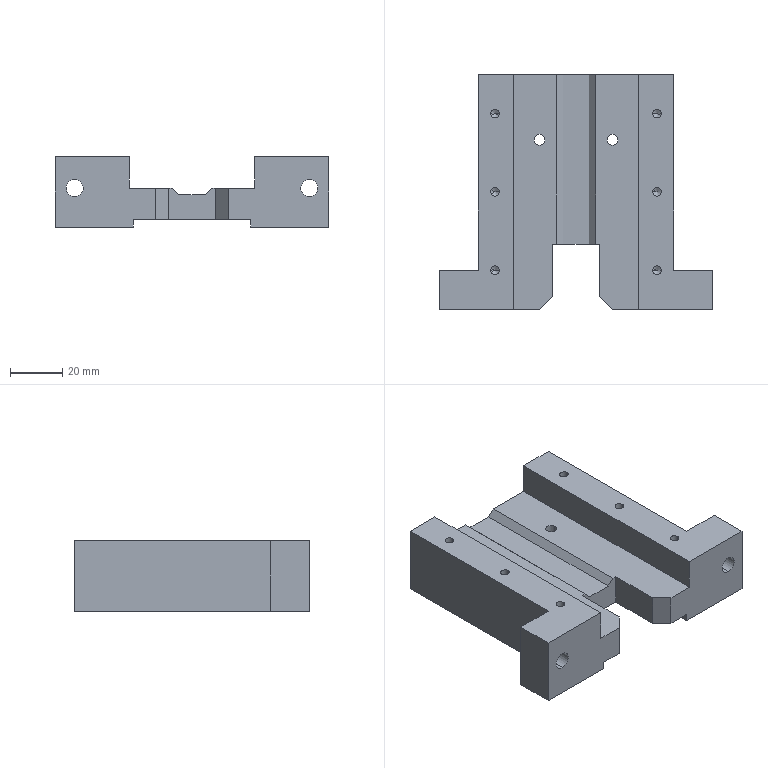Part | STEP file | detection slide seat--1 | 1 solid | 68 faces | box 105 x 90 x 27 mm | volume 120388 mm3 | plane 28 | cylinder 24 | cone 16 | commonest cylinder face diameters 3.3 x12 4.2 x8 6.5 x4